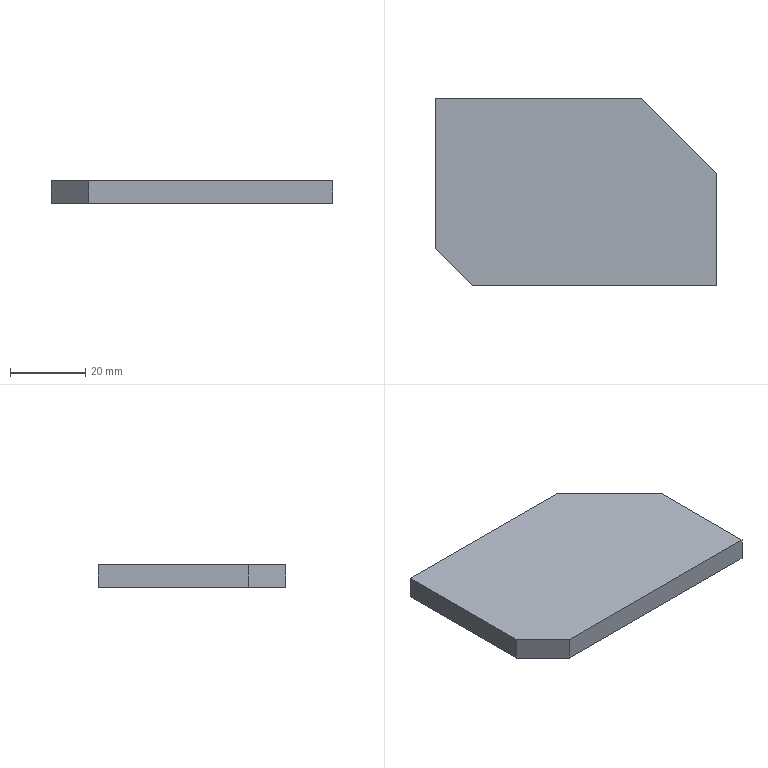Part | STEP file | [02]-10 | 1 solid | 8 faces | box 75 x 50 x 6 mm | volume 21000 mm3 | plane 8
STEP:
#1=CARTESIAN_POINT('',(0.,0.,0.));
#2=DIRECTION('',(0.,0.,1.));
#3=DIRECTION('',(1.,0.,0.));
#4=AXIS2_PLACEMENT_3D('',#1,#2,#3);
#5=CARTESIAN_POINT('',(75.,30.,6.));
#6=VERTEX_POINT('',#5);
#7=CARTESIAN_POINT('',(75.,0.,6.));
#8=VERTEX_POINT('',#7);
#9=CARTESIAN_POINT('',(75.,25.,6.));
#10=DIRECTION('',(0.,-1.,0.));
#11=VECTOR('',#10,1.);
#12=LINE('',#9,#11);
#13=CARTESIAN_POINT('',(37.5,25.,6.));
#14=DIRECTION('',(0.,0.,1.));
#15=DIRECTION('',(1.,0.,0.));
#16=AXIS2_PLACEMENT_3D('',#13,#14,#15);
#17=PLANE('',#16);
#18=CARTESIAN_POINT('',(37.5,0.));
#19=DIRECTION('',(0.,-1.));
#20=VECTOR('',#19,1.);
#21=LINE('',#18,#20);
#22=(GEOMETRIC_REPRESENTATION_CONTEXT(2)PARAMETRIC_REPRESENTATION_CONTEXT()REPRESENTATION_CONTEXT('',''));
#23=DEFINITIONAL_REPRESENTATION('',(#21),#22);
#24=PCURVE('',#17,#23);
#25=CARTESIAN_POINT('',(75.,25.,0.));
#26=DIRECTION('',(1.,0.,0.));
#27=DIRECTION('',(0.,0.,-1.));
#28=AXIS2_PLACEMENT_3D('',#25,#26,#27);
#29=PLANE('',#28);
#30=CARTESIAN_POINT('',(-6.,0.));
#31=DIRECTION('',(0.,-1.));
#32=VECTOR('',#31,1.);
#33=LINE('',#30,#32);
#34=(GEOMETRIC_REPRESENTATION_CONTEXT(2)PARAMETRIC_REPRESENTATION_CONTEXT()REPRESENTATION_CONTEXT('',''));
#35=DEFINITIONAL_REPRESENTATION('',(#33),#34);
#36=PCURVE('',#29,#35);
#37=SURFACE_CURVE('',#12,(#24,#36),.PCURVE_S1.);
#38=EDGE_CURVE('',#6,#8,#37,.T.);
#39=ORIENTED_EDGE('',*,*,#38,.F.);
#40=CARTESIAN_POINT('',(55.,50.,6.));
#41=VERTEX_POINT('',#40);
#42=CARTESIAN_POINT('',(58.75,46.25,6.));
#43=DIRECTION('',(-0.7071,0.7071,0.));
#44=VECTOR('',#43,1.);
#45=LINE('',#42,#44);
#46=CARTESIAN_POINT('',(21.25,21.25));
#47=DIRECTION('',(-0.7071,0.7071));
#48=VECTOR('',#47,1.);
#49=LINE('',#46,#48);
#50=(GEOMETRIC_REPRESENTATION_CONTEXT(2)PARAMETRIC_REPRESENTATION_CONTEXT()REPRESENTATION_CONTEXT('',''));
#51=DEFINITIONAL_REPRESENTATION('',(#49),#50);
#52=PCURVE('',#17,#51);
#53=CARTESIAN_POINT('',(75.,30.,0.));
#54=DIRECTION('',(-0.7071,-0.7071,0.));
#55=DIRECTION('',(0.,0.,1.));
#56=AXIS2_PLACEMENT_3D('',#53,#54,#55);
#57=PLANE('',#56);
#58=CARTESIAN_POINT('',(6.,22.981));
#59=DIRECTION('',(0.,1.));
#60=VECTOR('',#59,1.);
#61=LINE('',#58,#60);
#62=(GEOMETRIC_REPRESENTATION_CONTEXT(2)PARAMETRIC_REPRESENTATION_CONTEXT()REPRESENTATION_CONTEXT('',''));
#63=DEFINITIONAL_REPRESENTATION('',(#61),#62);
#64=PCURVE('',#57,#63);
#65=SURFACE_CURVE('',#45,(#52,#64),.PCURVE_S1.);
#66=EDGE_CURVE('',#6,#41,#65,.T.);
#67=ORIENTED_EDGE('',*,*,#66,.T.);
#68=CARTESIAN_POINT('',(0.,50.,6.));
#69=VERTEX_POINT('',#68);
#70=CARTESIAN_POINT('',(37.5,50.,6.));
#71=DIRECTION('',(1.,0.,0.));
#72=VECTOR('',#71,1.);
#73=LINE('',#70,#72);
#74=CARTESIAN_POINT('',(0.,25.));
#75=DIRECTION('',(1.,0.));
#76=VECTOR('',#75,1.);
#77=LINE('',#74,#76);
#78=(GEOMETRIC_REPRESENTATION_CONTEXT(2)PARAMETRIC_REPRESENTATION_CONTEXT()REPRESENTATION_CONTEXT('',''));
#79=DEFINITIONAL_REPRESENTATION('',(#77),#78);
#80=PCURVE('',#17,#79);
#81=CARTESIAN_POINT('',(37.5,50.,0.));
#82=DIRECTION('',(0.,1.,0.));
#83=DIRECTION('',(0.,0.,1.));
#84=AXIS2_PLACEMENT_3D('',#81,#82,#83);
#85=PLANE('',#84);
#86=CARTESIAN_POINT('',(6.,0.));
#87=DIRECTION('',(0.,1.));
#88=VECTOR('',#87,1.);
#89=LINE('',#86,#88);
#90=(GEOMETRIC_REPRESENTATION_CONTEXT(2)PARAMETRIC_REPRESENTATION_CONTEXT()REPRESENTATION_CONTEXT('',''));
#91=DEFINITIONAL_REPRESENTATION('',(#89),#90);
#92=PCURVE('',#85,#91);
#93=SURFACE_CURVE('',#73,(#80,#92),.PCURVE_S1.);
#94=EDGE_CURVE('',#69,#41,#93,.T.);
#95=ORIENTED_EDGE('',*,*,#94,.F.);
#96=CARTESIAN_POINT('',(0.,10.,6.));
#97=VERTEX_POINT('',#96);
#98=CARTESIAN_POINT('',(0.,25.,6.));
#99=DIRECTION('',(0.,1.,0.));
#100=VECTOR('',#99,1.);
#101=LINE('',#98,#100);
#102=CARTESIAN_POINT('',(-37.5,0.));
#103=DIRECTION('',(0.,1.));
#104=VECTOR('',#103,1.);
#105=LINE('',#102,#104);
#106=(GEOMETRIC_REPRESENTATION_CONTEXT(2)PARAMETRIC_REPRESENTATION_CONTEXT()REPRESENTATION_CONTEXT('',''));
#107=DEFINITIONAL_REPRESENTATION('',(#105),#106);
#108=PCURVE('',#17,#107);
#109=CARTESIAN_POINT('',(0.,25.,0.));
#110=DIRECTION('',(-1.,0.,0.));
#111=DIRECTION('',(0.,0.,1.));
#112=AXIS2_PLACEMENT_3D('',#109,#110,#111);
#113=PLANE('',#112);
#114=CARTESIAN_POINT('',(6.,0.));
#115=DIRECTION('',(0.,1.));
#116=VECTOR('',#115,1.);
#117=LINE('',#114,#116);
#118=(GEOMETRIC_REPRESENTATION_CONTEXT(2)PARAMETRIC_REPRESENTATION_CONTEXT()REPRESENTATION_CONTEXT('',''));
#119=DEFINITIONAL_REPRESENTATION('',(#117),#118);
#120=PCURVE('',#113,#119);
#121=SURFACE_CURVE('',#101,(#108,#120),.PCURVE_S1.);
#122=EDGE_CURVE('',#97,#69,#121,.T.);
#123=ORIENTED_EDGE('',*,*,#122,.F.);
#124=CARTESIAN_POINT('',(10.,0.,6.));
#125=VERTEX_POINT('',#124);
#126=CARTESIAN_POINT('',(11.25,-1.25,6.));
#127=DIRECTION('',(0.7071,-0.7071,0.));
#128=VECTOR('',#127,1.);
#129=LINE('',#126,#128);
#130=CARTESIAN_POINT('',(-26.25,-26.25));
#131=DIRECTION('',(0.7071,-0.7071));
#132=VECTOR('',#131,1.);
#133=LINE('',#130,#132);
#134=(GEOMETRIC_REPRESENTATION_CONTEXT(2)PARAMETRIC_REPRESENTATION_CONTEXT()REPRESENTATION_CONTEXT('',''));
#135=DEFINITIONAL_REPRESENTATION('',(#133),#134);
#136=PCURVE('',#17,#135);
#137=CARTESIAN_POINT('',(0.,10.,0.));
#138=DIRECTION('',(0.7071,0.7071,0.));
#139=DIRECTION('',(0.,0.,1.));
#140=AXIS2_PLACEMENT_3D('',#137,#138,#139);
#141=PLANE('',#140);
#142=CARTESIAN_POINT('',(6.,15.91));
#143=DIRECTION('',(0.,1.));
#144=VECTOR('',#143,1.);
#145=LINE('',#142,#144);
#146=(GEOMETRIC_REPRESENTATION_CONTEXT(2)PARAMETRIC_REPRESENTATION_CONTEXT()REPRESENTATION_CONTEXT('',''));
#147=DEFINITIONAL_REPRESENTATION('',(#145),#146);
#148=PCURVE('',#141,#147);
#149=SURFACE_CURVE('',#129,(#136,#148),.PCURVE_S1.);
#150=EDGE_CURVE('',#97,#125,#149,.T.);
#151=ORIENTED_EDGE('',*,*,#150,.T.);
#152=CARTESIAN_POINT('',(37.5,0.,6.));
#153=DIRECTION('',(-1.,0.,0.));
#154=VECTOR('',#153,1.);
#155=LINE('',#152,#154);
#156=CARTESIAN_POINT('',(0.,-25.));
#157=DIRECTION('',(-1.,0.));
#158=VECTOR('',#157,1.);
#159=LINE('',#156,#158);
#160=(GEOMETRIC_REPRESENTATION_CONTEXT(2)PARAMETRIC_REPRESENTATION_CONTEXT()REPRESENTATION_CONTEXT('',''));
#161=DEFINITIONAL_REPRESENTATION('',(#159),#160);
#162=PCURVE('',#17,#161);
#163=CARTESIAN_POINT('',(37.5,0.,0.));
#164=DIRECTION('',(0.,-1.,0.));
#165=DIRECTION('',(0.,0.,-1.));
#166=AXIS2_PLACEMENT_3D('',#163,#164,#165);
#167=PLANE('',#166);
#168=CARTESIAN_POINT('',(-6.,0.));
#169=DIRECTION('',(0.,-1.));
#170=VECTOR('',#169,1.);
#171=LINE('',#168,#170);
#172=(GEOMETRIC_REPRESENTATION_CONTEXT(2)PARAMETRIC_REPRESENTATION_CONTEXT()REPRESENTATION_CONTEXT('',''));
#173=DEFINITIONAL_REPRESENTATION('',(#171),#172);
#174=PCURVE('',#167,#173);
#175=SURFACE_CURVE('',#155,(#162,#174),.PCURVE_S1.);
#176=EDGE_CURVE('',#8,#125,#175,.T.);
#177=ORIENTED_EDGE('',*,*,#176,.F.);
#178=EDGE_LOOP('',(#39,#67,#95,#123,#151,#177));
#179=FACE_BOUND('',#178,.T.);
#180=ADVANCED_FACE('',(#179),#17,.T.);
#181=ORIENTED_EDGE('',*,*,#176,.T.);
#182=CARTESIAN_POINT('',(10.,0.,0.));
#183=VERTEX_POINT('',#182);
#184=CARTESIAN_POINT('',(10.,0.,0.));
#185=DIRECTION('',(0.,0.,-1.));
#186=VECTOR('',#185,1.);
#187=LINE('',#184,#186);
#188=CARTESIAN_POINT('',(0.,-27.5));
#189=DIRECTION('',(1.,0.));
#190=VECTOR('',#189,1.);
#191=LINE('',#188,#190);
#192=(GEOMETRIC_REPRESENTATION_CONTEXT(2)PARAMETRIC_REPRESENTATION_CONTEXT()REPRESENTATION_CONTEXT('',''));
#193=DEFINITIONAL_REPRESENTATION('',(#191),#192);
#194=PCURVE('',#167,#193);
#195=CARTESIAN_POINT('',(0.,14.142));
#196=DIRECTION('',(-1.,0.));
#197=VECTOR('',#196,1.);
#198=LINE('',#195,#197);
#199=(GEOMETRIC_REPRESENTATION_CONTEXT(2)PARAMETRIC_REPRESENTATION_CONTEXT()REPRESENTATION_CONTEXT('',''));
#200=DEFINITIONAL_REPRESENTATION('',(#198),#199);
#201=PCURVE('',#141,#200);
#202=SURFACE_CURVE('',#187,(#194,#201),.PCURVE_S1.);
#203=EDGE_CURVE('',#125,#183,#202,.T.);
#204=ORIENTED_EDGE('',*,*,#203,.T.);
#205=CARTESIAN_POINT('',(75.,0.,0.));
#206=VERTEX_POINT('',#205);
#207=CARTESIAN_POINT('',(37.5,0.,0.));
#208=DIRECTION('',(1.,0.,0.));
#209=VECTOR('',#208,1.);
#210=LINE('',#207,#209);
#211=CARTESIAN_POINT('',(0.,0.));
#212=DIRECTION('',(0.,1.));
#213=VECTOR('',#212,1.);
#214=LINE('',#211,#213);
#215=(GEOMETRIC_REPRESENTATION_CONTEXT(2)PARAMETRIC_REPRESENTATION_CONTEXT()REPRESENTATION_CONTEXT('',''));
#216=DEFINITIONAL_REPRESENTATION('',(#214),#215);
#217=PCURVE('',#167,#216);
#218=CARTESIAN_POINT('',(37.5,25.,0.));
#219=DIRECTION('',(0.,0.,-1.));
#220=DIRECTION('',(-1.,0.,0.));
#221=AXIS2_PLACEMENT_3D('',#218,#219,#220);
#222=PLANE('',#221);
#223=CARTESIAN_POINT('',(0.,-25.));
#224=DIRECTION('',(-1.,0.));
#225=VECTOR('',#224,1.);
#226=LINE('',#223,#225);
#227=(GEOMETRIC_REPRESENTATION_CONTEXT(2)PARAMETRIC_REPRESENTATION_CONTEXT()REPRESENTATION_CONTEXT('',''));
#228=DEFINITIONAL_REPRESENTATION('',(#226),#227);
#229=PCURVE('',#222,#228);
#230=SURFACE_CURVE('',#210,(#217,#229),.PCURVE_S1.);
#231=EDGE_CURVE('',#183,#206,#230,.T.);
#232=ORIENTED_EDGE('',*,*,#231,.T.);
#233=CARTESIAN_POINT('',(75.,0.,0.));
#234=DIRECTION('',(0.,0.,1.));
#235=VECTOR('',#234,1.);
#236=LINE('',#233,#235);
#237=CARTESIAN_POINT('',(0.,37.5));
#238=DIRECTION('',(-1.,0.));
#239=VECTOR('',#238,1.);
#240=LINE('',#237,#239);
#241=(GEOMETRIC_REPRESENTATION_CONTEXT(2)PARAMETRIC_REPRESENTATION_CONTEXT()REPRESENTATION_CONTEXT('',''));
#242=DEFINITIONAL_REPRESENTATION('',(#240),#241);
#243=PCURVE('',#167,#242);
#244=CARTESIAN_POINT('',(0.,-25.));
#245=DIRECTION('',(-1.,0.));
#246=VECTOR('',#245,1.);
#247=LINE('',#244,#246);
#248=(GEOMETRIC_REPRESENTATION_CONTEXT(2)PARAMETRIC_REPRESENTATION_CONTEXT()REPRESENTATION_CONTEXT('',''));
#249=DEFINITIONAL_REPRESENTATION('',(#247),#248);
#250=PCURVE('',#29,#249);
#251=SURFACE_CURVE('',#236,(#243,#250),.PCURVE_S1.);
#252=EDGE_CURVE('',#206,#8,#251,.T.);
#253=ORIENTED_EDGE('',*,*,#252,.T.);
#254=EDGE_LOOP('',(#181,#204,#232,#253));
#255=FACE_BOUND('',#254,.T.);
#256=ADVANCED_FACE('',(#255),#167,.T.);
#257=CARTESIAN_POINT('',(0.,50.,0.));
#258=VERTEX_POINT('',#257);
#259=CARTESIAN_POINT('',(0.,10.,0.));
#260=VERTEX_POINT('',#259);
#261=CARTESIAN_POINT('',(0.,25.,0.));
#262=DIRECTION('',(0.,-1.,0.));
#263=VECTOR('',#262,1.);
#264=LINE('',#261,#263);
#265=CARTESIAN_POINT('',(0.,0.));
#266=DIRECTION('',(0.,-1.));
#267=VECTOR('',#266,1.);
#268=LINE('',#265,#267);
#269=(GEOMETRIC_REPRESENTATION_CONTEXT(2)PARAMETRIC_REPRESENTATION_CONTEXT()REPRESENTATION_CONTEXT('',''));
#270=DEFINITIONAL_REPRESENTATION('',(#268),#269);
#271=PCURVE('',#113,#270);
#272=CARTESIAN_POINT('',(37.5,0.));
#273=DIRECTION('',(0.,-1.));
#274=VECTOR('',#273,1.);
#275=LINE('',#272,#274);
#276=(GEOMETRIC_REPRESENTATION_CONTEXT(2)PARAMETRIC_REPRESENTATION_CONTEXT()REPRESENTATION_CONTEXT('',''));
#277=DEFINITIONAL_REPRESENTATION('',(#275),#276);
#278=PCURVE('',#222,#277);
#279=SURFACE_CURVE('',#264,(#271,#278),.PCURVE_S1.);
#280=EDGE_CURVE('',#258,#260,#279,.T.);
#281=ORIENTED_EDGE('',*,*,#280,.T.);
#282=CARTESIAN_POINT('',(0.,10.,0.));
#283=DIRECTION('',(0.,0.,1.));
#284=VECTOR('',#283,1.);
#285=LINE('',#282,#284);
#286=CARTESIAN_POINT('',(0.,-15.));
#287=DIRECTION('',(1.,0.));
#288=VECTOR('',#287,1.);
#289=LINE('',#286,#288);
#290=(GEOMETRIC_REPRESENTATION_CONTEXT(2)PARAMETRIC_REPRESENTATION_CONTEXT()REPRESENTATION_CONTEXT('',''));
#291=DEFINITIONAL_REPRESENTATION('',(#289),#290);
#292=PCURVE('',#113,#291);
#293=CARTESIAN_POINT('',(0.,0.));
#294=DIRECTION('',(1.,0.));
#295=VECTOR('',#294,1.);
#296=LINE('',#293,#295);
#297=(GEOMETRIC_REPRESENTATION_CONTEXT(2)PARAMETRIC_REPRESENTATION_CONTEXT()REPRESENTATION_CONTEXT('',''));
#298=DEFINITIONAL_REPRESENTATION('',(#296),#297);
#299=PCURVE('',#141,#298);
#300=SURFACE_CURVE('',#285,(#292,#299),.PCURVE_S1.);
#301=EDGE_CURVE('',#260,#97,#300,.T.);
#302=ORIENTED_EDGE('',*,*,#301,.T.);
#303=ORIENTED_EDGE('',*,*,#122,.T.);
#304=CARTESIAN_POINT('',(0.,50.,0.));
#305=DIRECTION('',(0.,0.,1.));
#306=VECTOR('',#305,1.);
#307=LINE('',#304,#306);
#308=CARTESIAN_POINT('',(0.,25.));
#309=DIRECTION('',(1.,0.));
#310=VECTOR('',#309,1.);
#311=LINE('',#308,#310);
#312=(GEOMETRIC_REPRESENTATION_CONTEXT(2)PARAMETRIC_REPRESENTATION_CONTEXT()REPRESENTATION_CONTEXT('',''));
#313=DEFINITIONAL_REPRESENTATION('',(#311),#312);
#314=PCURVE('',#113,#313);
#315=CARTESIAN_POINT('',(0.,-37.5));
#316=DIRECTION('',(1.,0.));
#317=VECTOR('',#316,1.);
#318=LINE('',#315,#317);
#319=(GEOMETRIC_REPRESENTATION_CONTEXT(2)PARAMETRIC_REPRESENTATION_CONTEXT()REPRESENTATION_CONTEXT('',''));
#320=DEFINITIONAL_REPRESENTATION('',(#318),#319);
#321=PCURVE('',#85,#320);
#322=SURFACE_CURVE('',#307,(#314,#321),.PCURVE_S1.);
#323=EDGE_CURVE('',#258,#69,#322,.T.);
#324=ORIENTED_EDGE('',*,*,#323,.F.);
#325=EDGE_LOOP('',(#281,#302,#303,#324));
#326=FACE_BOUND('',#325,.T.);
#327=ADVANCED_FACE('',(#326),#113,.T.);
#328=ORIENTED_EDGE('',*,*,#94,.T.);
#329=CARTESIAN_POINT('',(55.,50.,0.));
#330=VERTEX_POINT('',#329);
#331=CARTESIAN_POINT('',(55.,50.,0.));
#332=DIRECTION('',(0.,0.,-1.));
#333=VECTOR('',#332,1.);
#334=LINE('',#331,#333);
#335=CARTESIAN_POINT('',(0.,17.5));
#336=DIRECTION('',(-1.,0.));
#337=VECTOR('',#336,1.);
#338=LINE('',#335,#337);
#339=(GEOMETRIC_REPRESENTATION_CONTEXT(2)PARAMETRIC_REPRESENTATION_CONTEXT()REPRESENTATION_CONTEXT('',''));
#340=DEFINITIONAL_REPRESENTATION('',(#338),#339);
#341=PCURVE('',#85,#340);
#342=CARTESIAN_POINT('',(0.,28.284));
#343=DIRECTION('',(-1.,0.));
#344=VECTOR('',#343,1.);
#345=LINE('',#342,#344);
#346=(GEOMETRIC_REPRESENTATION_CONTEXT(2)PARAMETRIC_REPRESENTATION_CONTEXT()REPRESENTATION_CONTEXT('',''));
#347=DEFINITIONAL_REPRESENTATION('',(#345),#346);
#348=PCURVE('',#57,#347);
#349=SURFACE_CURVE('',#334,(#341,#348),.PCURVE_S1.);
#350=EDGE_CURVE('',#41,#330,#349,.T.);
#351=ORIENTED_EDGE('',*,*,#350,.T.);
#352=CARTESIAN_POINT('',(37.5,50.,0.));
#353=DIRECTION('',(-1.,0.,0.));
#354=VECTOR('',#353,1.);
#355=LINE('',#352,#354);
#356=CARTESIAN_POINT('',(0.,0.));
#357=DIRECTION('',(0.,-1.));
#358=VECTOR('',#357,1.);
#359=LINE('',#356,#358);
#360=(GEOMETRIC_REPRESENTATION_CONTEXT(2)PARAMETRIC_REPRESENTATION_CONTEXT()REPRESENTATION_CONTEXT('',''));
#361=DEFINITIONAL_REPRESENTATION('',(#359),#360);
#362=PCURVE('',#85,#361);
#363=CARTESIAN_POINT('',(0.,25.));
#364=DIRECTION('',(1.,0.));
#365=VECTOR('',#364,1.);
#366=LINE('',#363,#365);
#367=(GEOMETRIC_REPRESENTATION_CONTEXT(2)PARAMETRIC_REPRESENTATION_CONTEXT()REPRESENTATION_CONTEXT('',''));
#368=DEFINITIONAL_REPRESENTATION('',(#366),#367);
#369=PCURVE('',#222,#368);
#370=SURFACE_CURVE('',#355,(#362,#369),.PCURVE_S1.);
#371=EDGE_CURVE('',#330,#258,#370,.T.);
#372=ORIENTED_EDGE('',*,*,#371,.T.);
#373=ORIENTED_EDGE('',*,*,#323,.T.);
#374=EDGE_LOOP('',(#328,#351,#372,#373));
#375=FACE_BOUND('',#374,.T.);
#376=ADVANCED_FACE('',(#375),#85,.T.);
#377=ORIENTED_EDGE('',*,*,#371,.F.);
#378=CARTESIAN_POINT('',(75.,30.,0.));
#379=VERTEX_POINT('',#378);
#380=CARTESIAN_POINT('',(58.75,46.25,0.));
#381=DIRECTION('',(0.7071,-0.7071,0.));
#382=VECTOR('',#381,1.);
#383=LINE('',#380,#382);
#384=CARTESIAN_POINT('',(-21.25,21.25));
#385=DIRECTION('',(-0.7071,-0.7071));
#386=VECTOR('',#385,1.);
#387=LINE('',#384,#386);
#388=(GEOMETRIC_REPRESENTATION_CONTEXT(2)PARAMETRIC_REPRESENTATION_CONTEXT()REPRESENTATION_CONTEXT('',''));
#389=DEFINITIONAL_REPRESENTATION('',(#387),#388);
#390=PCURVE('',#222,#389);
#391=CARTESIAN_POINT('',(0.,22.981));
#392=DIRECTION('',(0.,-1.));
#393=VECTOR('',#392,1.);
#394=LINE('',#391,#393);
#395=(GEOMETRIC_REPRESENTATION_CONTEXT(2)PARAMETRIC_REPRESENTATION_CONTEXT()REPRESENTATION_CONTEXT('',''));
#396=DEFINITIONAL_REPRESENTATION('',(#394),#395);
#397=PCURVE('',#57,#396);
#398=SURFACE_CURVE('',#383,(#390,#397),.PCURVE_S1.);
#399=EDGE_CURVE('',#330,#379,#398,.T.);
#400=ORIENTED_EDGE('',*,*,#399,.T.);
#401=CARTESIAN_POINT('',(75.,25.,0.));
#402=DIRECTION('',(0.,1.,0.));
#403=VECTOR('',#402,1.);
#404=LINE('',#401,#403);
#405=CARTESIAN_POINT('',(-37.5,0.));
#406=DIRECTION('',(0.,1.));
#407=VECTOR('',#406,1.);
#408=LINE('',#405,#407);
#409=(GEOMETRIC_REPRESENTATION_CONTEXT(2)PARAMETRIC_REPRESENTATION_CONTEXT()REPRESENTATION_CONTEXT('',''));
#410=DEFINITIONAL_REPRESENTATION('',(#408),#409);
#411=PCURVE('',#222,#410);
#412=CARTESIAN_POINT('',(0.,0.));
#413=DIRECTION('',(0.,1.));
#414=VECTOR('',#413,1.);
#415=LINE('',#412,#414);
#416=(GEOMETRIC_REPRESENTATION_CONTEXT(2)PARAMETRIC_REPRESENTATION_CONTEXT()REPRESENTATION_CONTEXT('',''));
#417=DEFINITIONAL_REPRESENTATION('',(#415),#416);
#418=PCURVE('',#29,#417);
#419=SURFACE_CURVE('',#404,(#411,#418),.PCURVE_S1.);
#420=EDGE_CURVE('',#206,#379,#419,.T.);
#421=ORIENTED_EDGE('',*,*,#420,.F.);
#422=ORIENTED_EDGE('',*,*,#231,.F.);
#423=CARTESIAN_POINT('',(11.25,-1.25,0.));
#424=DIRECTION('',(-0.7071,0.7071,0.));
#425=VECTOR('',#424,1.);
#426=LINE('',#423,#425);
#427=CARTESIAN_POINT('',(26.25,-26.25));
#428=DIRECTION('',(0.7071,0.7071));
#429=VECTOR('',#428,1.);
#430=LINE('',#427,#429);
#431=(GEOMETRIC_REPRESENTATION_CONTEXT(2)PARAMETRIC_REPRESENTATION_CONTEXT()REPRESENTATION_CONTEXT('',''));
#432=DEFINITIONAL_REPRESENTATION('',(#430),#431);
#433=PCURVE('',#222,#432);
#434=CARTESIAN_POINT('',(0.,15.91));
#435=DIRECTION('',(0.,-1.));
#436=VECTOR('',#435,1.);
#437=LINE('',#434,#436);
#438=(GEOMETRIC_REPRESENTATION_CONTEXT(2)PARAMETRIC_REPRESENTATION_CONTEXT()REPRESENTATION_CONTEXT('',''));
#439=DEFINITIONAL_REPRESENTATION('',(#437),#438);
#440=PCURVE('',#141,#439);
#441=SURFACE_CURVE('',#426,(#433,#440),.PCURVE_S1.);
#442=EDGE_CURVE('',#183,#260,#441,.T.);
#443=ORIENTED_EDGE('',*,*,#442,.T.);
#444=ORIENTED_EDGE('',*,*,#280,.F.);
#445=EDGE_LOOP('',(#377,#400,#421,#422,#443,#444));
#446=FACE_BOUND('',#445,.T.);
#447=ADVANCED_FACE('',(#446),#222,.T.);
#448=ORIENTED_EDGE('',*,*,#420,.T.);
#449=CARTESIAN_POINT('',(75.,30.,0.));
#450=DIRECTION('',(0.,0.,1.));
#451=VECTOR('',#450,1.);
#452=LINE('',#449,#451);
#453=CARTESIAN_POINT('',(0.,5.));
#454=DIRECTION('',(-1.,0.));
#455=VECTOR('',#454,1.);
#456=LINE('',#453,#455);
#457=(GEOMETRIC_REPRESENTATION_CONTEXT(2)PARAMETRIC_REPRESENTATION_CONTEXT()REPRESENTATION_CONTEXT('',''));
#458=DEFINITIONAL_REPRESENTATION('',(#456),#457);
#459=PCURVE('',#29,#458);
#460=CARTESIAN_POINT('',(0.,0.));
#461=DIRECTION('',(1.,0.));
#462=VECTOR('',#461,1.);
#463=LINE('',#460,#462);
#464=(GEOMETRIC_REPRESENTATION_CONTEXT(2)PARAMETRIC_REPRESENTATION_CONTEXT()REPRESENTATION_CONTEXT('',''));
#465=DEFINITIONAL_REPRESENTATION('',(#463),#464);
#466=PCURVE('',#57,#465);
#467=SURFACE_CURVE('',#452,(#459,#466),.PCURVE_S1.);
#468=EDGE_CURVE('',#379,#6,#467,.T.);
#469=ORIENTED_EDGE('',*,*,#468,.T.);
#470=ORIENTED_EDGE('',*,*,#38,.T.);
#471=ORIENTED_EDGE('',*,*,#252,.F.);
#472=EDGE_LOOP('',(#448,#469,#470,#471));
#473=FACE_BOUND('',#472,.T.);
#474=ADVANCED_FACE('',(#473),#29,.T.);
#475=ORIENTED_EDGE('',*,*,#442,.F.);
#476=ORIENTED_EDGE('',*,*,#203,.F.);
#477=ORIENTED_EDGE('',*,*,#150,.F.);
#478=ORIENTED_EDGE('',*,*,#301,.F.);
#479=EDGE_LOOP('',(#475,#476,#477,#478));
#480=FACE_BOUND('',#479,.T.);
#481=ADVANCED_FACE('',(#480),#141,.F.);
#482=ORIENTED_EDGE('',*,*,#399,.F.);
#483=ORIENTED_EDGE('',*,*,#350,.F.);
#484=ORIENTED_EDGE('',*,*,#66,.F.);
#485=ORIENTED_EDGE('',*,*,#468,.F.);
#486=EDGE_LOOP('',(#482,#483,#484,#485));
#487=FACE_BOUND('',#486,.T.);
#488=ADVANCED_FACE('',(#487),#57,.F.);
#489=CLOSED_SHELL('',(#180,#256,#327,#376,#447,#474,#481,#488));
#490=MANIFOLD_SOLID_BREP('',#489);
#491=(LENGTH_UNIT()NAMED_UNIT(*)SI_UNIT(.MILLI.,.METRE.));
#492=UNCERTAINTY_MEASURE_WITH_UNIT(LENGTH_MEASURE(0.0000001),#491,'','');
#493=(NAMED_UNIT(*)PLANE_ANGLE_UNIT()SI_UNIT($,.RADIAN.));
#494=(NAMED_UNIT(*)SI_UNIT($,.STERADIAN.)SOLID_ANGLE_UNIT());
#495=(GEOMETRIC_REPRESENTATION_CONTEXT(3)GLOBAL_UNCERTAINTY_ASSIGNED_CONTEXT((#492))GLOBAL_UNIT_ASSIGNED_CONTEXT((#491,#493,#494))REPRESENTATION_CONTEXT('',''));
#496=ADVANCED_BREP_SHAPE_REPRESENTATION('',(#4,#490),#495);